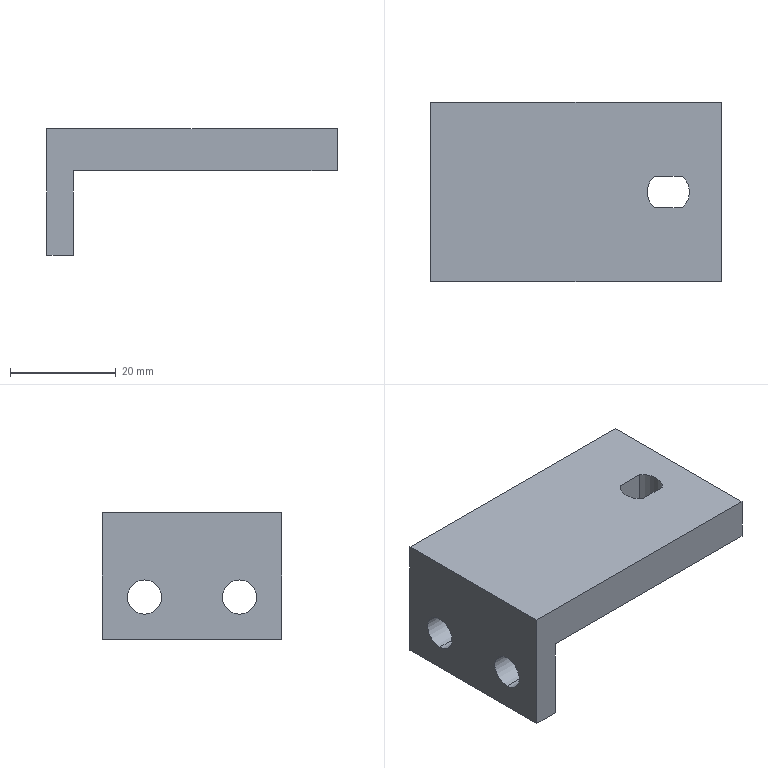Part | STEP file | 8xs043021 | 1 solid | 17 faces | box 55 x 34 x 24 mm | volume 17004 mm3 | plane 10 | cylinder 7 | commonest cylinder face diameters 6.5 x4 8 x3
STEP:
#1=CARTESIAN_POINT('',(0.,0.,0.));
#2=DIRECTION('',(0.,0.,1.));
#3=DIRECTION('',(1.,0.,0.));
#4=AXIS2_PLACEMENT_3D('',#1,#2,#3);
#5=CARTESIAN_POINT('',(14.854,3.,24.));
#6=VERTEX_POINT('',#5);
#7=CARTESIAN_POINT('',(14.854,3.,16.));
#8=VERTEX_POINT('',#7);
#9=CARTESIAN_POINT('',(14.854,3.,26.));
#10=DIRECTION('',(0.,0.,-1.));
#11=VECTOR('',#10,1.);
#12=LINE('',#9,#11);
#13=CARTESIAN_POINT('',(17.5,0.,26.));
#14=DIRECTION('',(0.,0.,-1.));
#15=DIRECTION('',(-1.,0.,0.));
#16=AXIS2_PLACEMENT_3D('',#13,#14,#15);
#17=CYLINDRICAL_SURFACE('',#16,4.);
#18=CARTESIAN_POINT('',(0.8481,0.));
#19=DIRECTION('',(0.,1.));
#20=VECTOR('',#19,1.);
#21=LINE('',#18,#20);
#22=(GEOMETRIC_REPRESENTATION_CONTEXT(2)PARAMETRIC_REPRESENTATION_CONTEXT()REPRESENTATION_CONTEXT('',''));
#23=DEFINITIONAL_REPRESENTATION('',(#21),#22);
#24=PCURVE('',#17,#23);
#25=CARTESIAN_POINT('',(20.146,3.,26.));
#26=DIRECTION('',(0.,1.,0.));
#27=DIRECTION('',(-1.,0.,0.));
#28=AXIS2_PLACEMENT_3D('',#25,#26,#27);
#29=PLANE('',#28);
#30=CARTESIAN_POINT('',(5.292,0.));
#31=DIRECTION('',(0.,-1.));
#32=VECTOR('',#31,1.);
#33=LINE('',#30,#32);
#34=(GEOMETRIC_REPRESENTATION_CONTEXT(2)PARAMETRIC_REPRESENTATION_CONTEXT()REPRESENTATION_CONTEXT('',''));
#35=DEFINITIONAL_REPRESENTATION('',(#33),#34);
#36=PCURVE('',#29,#35);
#37=SURFACE_CURVE('',#12,(#24,#36),.PCURVE_S1.);
#38=EDGE_CURVE('',#6,#8,#37,.T.);
#39=ORIENTED_EDGE('',*,*,#38,.T.);
#40=CARTESIAN_POINT('',(13.5,0.,16.));
#41=VERTEX_POINT('',#40);
#42=CARTESIAN_POINT('',(17.5,0.,16.));
#43=DIRECTION('',(0.,0.,-1.));
#44=DIRECTION('',(-1.,0.,0.));
#45=AXIS2_PLACEMENT_3D('',#42,#43,#44);
#46=CIRCLE('',#45,4.);
#47=CARTESIAN_POINT('',(0.,10.));
#48=DIRECTION('',(1.,0.));
#49=VECTOR('',#48,1.);
#50=LINE('',#47,#49);
#51=(GEOMETRIC_REPRESENTATION_CONTEXT(2)PARAMETRIC_REPRESENTATION_CONTEXT()REPRESENTATION_CONTEXT('',''));
#52=DEFINITIONAL_REPRESENTATION('',(#50),#51);
#53=PCURVE('',#17,#52);
#54=CARTESIAN_POINT('',(27.5,-17.,16.));
#55=DIRECTION('',(0.,0.,1.));
#56=DIRECTION('',(1.,0.,0.));
#57=AXIS2_PLACEMENT_3D('',#54,#55,#56);
#58=PLANE('',#57);
#59=CARTESIAN_POINT('',(-14.,17.));
#60=CARTESIAN_POINT('',(-14.,23.928));
#61=CARTESIAN_POINT('',(-8.,20.464));
#62=CARTESIAN_POINT('',(-2.,17.));
#63=CARTESIAN_POINT('',(-8.,13.536));
#64=CARTESIAN_POINT('',(-14.,10.072));
#65=CARTESIAN_POINT('',(-14.,17.));
#66=(BOUNDED_CURVE()B_SPLINE_CURVE(2,(#59,#60,#61,#62,#63,#64,#65),.UNSPECIFIED.,.T.,.F.)B_SPLINE_CURVE_WITH_KNOTS((1,2,2,2,2,1),(-2.094,0.,2.094,4.189,6.283,8.378),.UNSPECIFIED.)CURVE()GEOMETRIC_REPRESENTATION_ITEM()RATIONAL_B_SPLINE_CURVE((1.,0.5,1.,0.5,1.,0.5,1.))REPRESENTATION_ITEM(''));
#67=(GEOMETRIC_REPRESENTATION_CONTEXT(2)PARAMETRIC_REPRESENTATION_CONTEXT()REPRESENTATION_CONTEXT('',''));
#68=DEFINITIONAL_REPRESENTATION('',(#66),#67);
#69=PCURVE('',#58,#68);
#70=SURFACE_CURVE('',#46,(#53,#69),.PCURVE_S1.);
#71=EDGE_CURVE('',#41,#8,#70,.T.);
#72=ORIENTED_EDGE('',*,*,#71,.F.);
#73=CARTESIAN_POINT('',(13.5,0.,24.));
#74=VERTEX_POINT('',#73);
#75=CARTESIAN_POINT('',(13.5,0.,26.));
#76=DIRECTION('',(0.,0.,-1.));
#77=VECTOR('',#76,1.);
#78=LINE('',#75,#77);
#79=CARTESIAN_POINT('',(0.,0.));
#80=DIRECTION('',(0.,1.));
#81=VECTOR('',#80,1.);
#82=LINE('',#79,#81);
#83=(GEOMETRIC_REPRESENTATION_CONTEXT(2)PARAMETRIC_REPRESENTATION_CONTEXT()REPRESENTATION_CONTEXT('',''));
#84=DEFINITIONAL_REPRESENTATION('',(#82),#83);
#85=PCURVE('',#17,#84);
#86=CARTESIAN_POINT('',(17.5,0.,26.));
#87=DIRECTION('',(0.,0.,-1.));
#88=DIRECTION('',(-1.,0.,0.));
#89=AXIS2_PLACEMENT_3D('',#86,#87,#88);
#90=CYLINDRICAL_SURFACE('',#89,4.);
#91=CARTESIAN_POINT('',(6.283,0.));
#92=DIRECTION('',(0.,1.));
#93=VECTOR('',#92,1.);
#94=LINE('',#91,#93);
#95=(GEOMETRIC_REPRESENTATION_CONTEXT(2)PARAMETRIC_REPRESENTATION_CONTEXT()REPRESENTATION_CONTEXT('',''));
#96=DEFINITIONAL_REPRESENTATION('',(#94),#95);
#97=PCURVE('',#90,#96);
#98=SURFACE_CURVE('',#78,(#85,#97),.PCURVE_S1.);
#99=EDGE_CURVE('',#74,#41,#98,.T.);
#100=ORIENTED_EDGE('',*,*,#99,.F.);
#101=CARTESIAN_POINT('',(17.5,0.,24.));
#102=DIRECTION('',(0.,0.,-1.));
#103=DIRECTION('',(-1.,0.,0.));
#104=AXIS2_PLACEMENT_3D('',#101,#102,#103);
#105=CIRCLE('',#104,4.);
#106=CARTESIAN_POINT('',(0.,2.));
#107=DIRECTION('',(1.,0.));
#108=VECTOR('',#107,1.);
#109=LINE('',#106,#108);
#110=(GEOMETRIC_REPRESENTATION_CONTEXT(2)PARAMETRIC_REPRESENTATION_CONTEXT()REPRESENTATION_CONTEXT('',''));
#111=DEFINITIONAL_REPRESENTATION('',(#109),#110);
#112=PCURVE('',#17,#111);
#113=CARTESIAN_POINT('',(-27.5,-17.,24.));
#114=DIRECTION('',(0.,0.,-1.));
#115=DIRECTION('',(-1.,0.,0.));
#116=AXIS2_PLACEMENT_3D('',#113,#114,#115);
#117=PLANE('',#116);
#118=CARTESIAN_POINT('',(-45.,17.));
#119=DIRECTION('',(1.,0.));
#120=AXIS2_PLACEMENT_2D('',#118,#119);
#121=CIRCLE('',#120,4.);
#122=(GEOMETRIC_REPRESENTATION_CONTEXT(2)PARAMETRIC_REPRESENTATION_CONTEXT()REPRESENTATION_CONTEXT('',''));
#123=DEFINITIONAL_REPRESENTATION('',(#121),#122);
#124=PCURVE('',#117,#123);
#125=SURFACE_CURVE('',#105,(#112,#124),.PCURVE_S1.);
#126=EDGE_CURVE('',#74,#6,#125,.T.);
#127=ORIENTED_EDGE('',*,*,#126,.T.);
#128=EDGE_LOOP('',(#39,#72,#100,#127));
#129=FACE_BOUND('',#128,.F.);
#130=ADVANCED_FACE('',(#129),#17,.F.);
#131=CARTESIAN_POINT('',(-27.5,-9.,4.75));
#132=VERTEX_POINT('',#131);
#133=CARTESIAN_POINT('',(-22.5,-9.,4.75));
#134=VERTEX_POINT('',#133);
#135=CARTESIAN_POINT('',(-32.5,-9.,4.75));
#136=DIRECTION('',(1.,0.,0.));
#137=VECTOR('',#136,1.);
#138=LINE('',#135,#137);
#139=CARTESIAN_POINT('',(-32.5,-9.,8.));
#140=DIRECTION('',(1.,0.,0.));
#141=DIRECTION('',(0.,0.,-1.));
#142=AXIS2_PLACEMENT_3D('',#139,#140,#141);
#143=CYLINDRICAL_SURFACE('',#142,3.25);
#144=CARTESIAN_POINT('',(6.283,5.));
#145=CARTESIAN_POINT('',(6.283,5.076));
#146=CARTESIAN_POINT('',(6.283,5.227));
#147=CARTESIAN_POINT('',(6.283,5.455));
#148=CARTESIAN_POINT('',(6.283,5.682));
#149=CARTESIAN_POINT('',(6.283,5.909));
#150=CARTESIAN_POINT('',(6.283,6.136));
#151=CARTESIAN_POINT('',(6.283,6.364));
#152=CARTESIAN_POINT('',(6.283,6.591));
#153=CARTESIAN_POINT('',(6.283,6.818));
#154=CARTESIAN_POINT('',(6.283,7.045));
#155=CARTESIAN_POINT('',(6.283,7.273));
#156=CARTESIAN_POINT('',(6.283,7.5));
#157=CARTESIAN_POINT('',(6.283,7.727));
#158=CARTESIAN_POINT('',(6.283,7.955));
#159=CARTESIAN_POINT('',(6.283,8.182));
#160=CARTESIAN_POINT('',(6.283,8.409));
#161=CARTESIAN_POINT('',(6.283,8.636));
#162=CARTESIAN_POINT('',(6.283,8.864));
#163=CARTESIAN_POINT('',(6.283,9.091));
#164=CARTESIAN_POINT('',(6.283,9.318));
#165=CARTESIAN_POINT('',(6.283,9.545));
#166=CARTESIAN_POINT('',(6.283,9.773));
#167=CARTESIAN_POINT('',(6.283,9.924));
#168=CARTESIAN_POINT('',(6.283,10.));
#169=B_SPLINE_CURVE_WITH_KNOTS('',3,(#144,#145,#146,#147,#148,#149,#150,#151,#152,#153,#154,#155,#156,#157,#158,#159,#160,#161,#162,#163,#164,#165,#166,#167,#168),.UNSPECIFIED.,.F.,.F.,(4,1,1,1,1,1,1,1,1,1,1,1,1,1,1,1,1,1,1,1,1,1,4),(5.,5.227,5.455,5.682,5.909,6.136,6.364,6.591,6.818,7.045,7.273,7.5,7.727,7.955,8.182,8.409,8.636,8.864,9.091,9.318,9.545,9.773,10.),.QUASI_UNIFORM_KNOTS.);
#170=(GEOMETRIC_REPRESENTATION_CONTEXT(2)PARAMETRIC_REPRESENTATION_CONTEXT()REPRESENTATION_CONTEXT('',''));
#171=DEFINITIONAL_REPRESENTATION('',(#169),#170);
#172=PCURVE('',#143,#171);
#173=CARTESIAN_POINT('',(-32.5,-9.,8.));
#174=DIRECTION('',(1.,0.,0.));
#175=DIRECTION('',(0.,0.,-1.));
#176=AXIS2_PLACEMENT_3D('',#173,#174,#175);
#177=CYLINDRICAL_SURFACE('',#176,3.25);
#178=CARTESIAN_POINT('',(0.,0.));
#179=DIRECTION('',(0.,1.));
#180=VECTOR('',#179,1.);
#181=LINE('',#178,#180);
#182=(GEOMETRIC_REPRESENTATION_CONTEXT(2)PARAMETRIC_REPRESENTATION_CONTEXT()REPRESENTATION_CONTEXT('',''));
#183=DEFINITIONAL_REPRESENTATION('',(#181),#182);
#184=PCURVE('',#177,#183);
#185=SURFACE_CURVE('',#138,(#172,#184),.PCURVE_S1.);
#186=EDGE_CURVE('',#132,#134,#185,.T.);
#187=ORIENTED_EDGE('',*,*,#186,.T.);
#188=CARTESIAN_POINT('',(-22.5,-9.,11.25));
#189=VERTEX_POINT('',#188);
#190=CARTESIAN_POINT('',(-22.5,-9.,8.));
#191=DIRECTION('',(1.,0.,0.));
#192=DIRECTION('',(0.,0.,-1.));
#193=AXIS2_PLACEMENT_3D('',#190,#191,#192);
#194=CIRCLE('',#193,3.25);
#195=CARTESIAN_POINT('',(0.,10.));
#196=DIRECTION('',(1.,0.));
#197=VECTOR('',#196,1.);
#198=LINE('',#195,#197);
#199=(GEOMETRIC_REPRESENTATION_CONTEXT(2)PARAMETRIC_REPRESENTATION_CONTEXT()REPRESENTATION_CONTEXT('',''));
#200=DEFINITIONAL_REPRESENTATION('',(#198),#199);
#201=PCURVE('',#143,#200);
#202=CARTESIAN_POINT('',(-22.5,-17.,0.));
#203=DIRECTION('',(-1.,0.,0.));
#204=DIRECTION('',(0.,0.,1.));
#205=AXIS2_PLACEMENT_3D('',#202,#203,#204);
#206=PLANE('',#205);
#207=CARTESIAN_POINT('',(4.75,8.));
#208=CARTESIAN_POINT('',(4.75,13.629));
#209=CARTESIAN_POINT('',(9.625,10.815));
#210=CARTESIAN_POINT('',(14.5,8.));
#211=CARTESIAN_POINT('',(9.625,5.185));
#212=CARTESIAN_POINT('',(4.75,2.371));
#213=CARTESIAN_POINT('',(4.75,8.));
#214=(BOUNDED_CURVE()B_SPLINE_CURVE(2,(#207,#208,#209,#210,#211,#212,#213),.UNSPECIFIED.,.T.,.F.)B_SPLINE_CURVE_WITH_KNOTS((1,2,2,2,2,1),(-2.094,0.,2.094,4.189,6.283,8.378),.UNSPECIFIED.)CURVE()GEOMETRIC_REPRESENTATION_ITEM()RATIONAL_B_SPLINE_CURVE((1.,0.5,1.,0.5,1.,0.5,1.))REPRESENTATION_ITEM(''));
#215=(GEOMETRIC_REPRESENTATION_CONTEXT(2)PARAMETRIC_REPRESENTATION_CONTEXT()REPRESENTATION_CONTEXT('',''));
#216=DEFINITIONAL_REPRESENTATION('',(#214),#215);
#217=PCURVE('',#206,#216);
#218=SURFACE_CURVE('',#194,(#201,#217),.PCURVE_S1.);
#219=EDGE_CURVE('',#189,#134,#218,.T.);
#220=ORIENTED_EDGE('',*,*,#219,.F.);
#221=CARTESIAN_POINT('',(-27.5,-9.,11.25));
#222=VERTEX_POINT('',#221);
#223=CARTESIAN_POINT('',(-32.5,-9.,11.25));
#224=DIRECTION('',(1.,0.,0.));
#225=VECTOR('',#224,1.);
#226=LINE('',#223,#225);
#227=CARTESIAN_POINT('',(3.142,0.));
#228=DIRECTION('',(0.,1.));
#229=VECTOR('',#228,1.);
#230=LINE('',#227,#229);
#231=(GEOMETRIC_REPRESENTATION_CONTEXT(2)PARAMETRIC_REPRESENTATION_CONTEXT()REPRESENTATION_CONTEXT('',''));
#232=DEFINITIONAL_REPRESENTATION('',(#230),#231);
#233=PCURVE('',#143,#232);
#234=CARTESIAN_POINT('',(3.142,0.));
#235=DIRECTION('',(0.,1.));
#236=VECTOR('',#235,1.);
#237=LINE('',#234,#236);
#238=(GEOMETRIC_REPRESENTATION_CONTEXT(2)PARAMETRIC_REPRESENTATION_CONTEXT()REPRESENTATION_CONTEXT('',''));
#239=DEFINITIONAL_REPRESENTATION('',(#237),#238);
#240=PCURVE('',#177,#239);
#241=SURFACE_CURVE('',#226,(#233,#240),.PCURVE_S1.);
#242=EDGE_CURVE('',#222,#189,#241,.T.);
#243=ORIENTED_EDGE('',*,*,#242,.F.);
#244=CARTESIAN_POINT('',(-27.5,-9.,8.));
#245=DIRECTION('',(1.,0.,0.));
#246=DIRECTION('',(0.,1.,0.));
#247=AXIS2_PLACEMENT_3D('',#244,#245,#246);
#248=CIRCLE('',#247,3.25);
#249=CARTESIAN_POINT('',(1.571,5.));
#250=DIRECTION('',(1.,0.));
#251=VECTOR('',#250,1.);
#252=LINE('',#249,#251);
#253=(GEOMETRIC_REPRESENTATION_CONTEXT(2)PARAMETRIC_REPRESENTATION_CONTEXT()REPRESENTATION_CONTEXT('',''));
#254=DEFINITIONAL_REPRESENTATION('',(#252),#253);
#255=PCURVE('',#143,#254);
#256=CARTESIAN_POINT('',(-27.5,17.,24.));
#257=DIRECTION('',(1.,0.,0.));
#258=DIRECTION('',(0.,1.,0.));
#259=AXIS2_PLACEMENT_3D('',#256,#257,#258);
#260=PLANE('',#259);
#261=CARTESIAN_POINT('',(-26.,-16.));
#262=DIRECTION('',(1.,0.));
#263=AXIS2_PLACEMENT_2D('',#261,#262);
#264=CIRCLE('',#263,3.25);
#265=(GEOMETRIC_REPRESENTATION_CONTEXT(2)PARAMETRIC_REPRESENTATION_CONTEXT()REPRESENTATION_CONTEXT('',''));
#266=DEFINITIONAL_REPRESENTATION('',(#264),#265);
#267=PCURVE('',#260,#266);
#268=SURFACE_CURVE('',#248,(#255,#267),.PCURVE_S1.);
#269=EDGE_CURVE('',#222,#132,#268,.T.);
#270=ORIENTED_EDGE('',*,*,#269,.T.);
#271=EDGE_LOOP('',(#187,#220,#243,#270));
#272=FACE_BOUND('',#271,.F.);
#273=ADVANCED_FACE('',(#272),#143,.F.);
#274=CARTESIAN_POINT('',(-27.5,9.,4.75));
#275=VERTEX_POINT('',#274);
#276=CARTESIAN_POINT('',(-22.5,9.,4.75));
#277=VERTEX_POINT('',#276);
#278=CARTESIAN_POINT('',(-32.5,9.,4.75));
#279=DIRECTION('',(1.,0.,0.));
#280=VECTOR('',#279,1.);
#281=LINE('',#278,#280);
#282=CARTESIAN_POINT('',(-32.5,9.,8.));
#283=DIRECTION('',(1.,0.,0.));
#284=DIRECTION('',(0.,0.,-1.));
#285=AXIS2_PLACEMENT_3D('',#282,#283,#284);
#286=CYLINDRICAL_SURFACE('',#285,3.25);
#287=CARTESIAN_POINT('',(6.283,5.));
#288=CARTESIAN_POINT('',(6.283,5.076));
#289=CARTESIAN_POINT('',(6.283,5.227));
#290=CARTESIAN_POINT('',(6.283,5.455));
#291=CARTESIAN_POINT('',(6.283,5.682));
#292=CARTESIAN_POINT('',(6.283,5.909));
#293=CARTESIAN_POINT('',(6.283,6.136));
#294=CARTESIAN_POINT('',(6.283,6.364));
#295=CARTESIAN_POINT('',(6.283,6.591));
#296=CARTESIAN_POINT('',(6.283,6.818));
#297=CARTESIAN_POINT('',(6.283,7.045));
#298=CARTESIAN_POINT('',(6.283,7.273));
#299=CARTESIAN_POINT('',(6.283,7.5));
#300=CARTESIAN_POINT('',(6.283,7.727));
#301=CARTESIAN_POINT('',(6.283,7.955));
#302=CARTESIAN_POINT('',(6.283,8.182));
#303=CARTESIAN_POINT('',(6.283,8.409));
#304=CARTESIAN_POINT('',(6.283,8.636));
#305=CARTESIAN_POINT('',(6.283,8.864));
#306=CARTESIAN_POINT('',(6.283,9.091));
#307=CARTESIAN_POINT('',(6.283,9.318));
#308=CARTESIAN_POINT('',(6.283,9.545));
#309=CARTESIAN_POINT('',(6.283,9.773));
#310=CARTESIAN_POINT('',(6.283,9.924));
#311=CARTESIAN_POINT('',(6.283,10.));
#312=B_SPLINE_CURVE_WITH_KNOTS('',3,(#287,#288,#289,#290,#291,#292,#293,#294,#295,#296,#297,#298,#299,#300,#301,#302,#303,#304,#305,#306,#307,#308,#309,#310,#311),.UNSPECIFIED.,.F.,.F.,(4,1,1,1,1,1,1,1,1,1,1,1,1,1,1,1,1,1,1,1,1,1,4),(5.,5.227,5.455,5.682,5.909,6.136,6.364,6.591,6.818,7.045,7.273,7.5,7.727,7.955,8.182,8.409,8.636,8.864,9.091,9.318,9.545,9.773,10.),.QUASI_UNIFORM_KNOTS.);
#313=(GEOMETRIC_REPRESENTATION_CONTEXT(2)PARAMETRIC_REPRESENTATION_CONTEXT()REPRESENTATION_CONTEXT('',''));
#314=DEFINITIONAL_REPRESENTATION('',(#312),#313);
#315=PCURVE('',#286,#314);
#316=CARTESIAN_POINT('',(-32.5,9.,8.));
#317=DIRECTION('',(1.,0.,0.));
#318=DIRECTION('',(0.,0.,-1.));
#319=AXIS2_PLACEMENT_3D('',#316,#317,#318);
#320=CYLINDRICAL_SURFACE('',#319,3.25);
#321=CARTESIAN_POINT('',(0.,0.));
#322=DIRECTION('',(0.,1.));
#323=VECTOR('',#322,1.);
#324=LINE('',#321,#323);
#325=(GEOMETRIC_REPRESENTATION_CONTEXT(2)PARAMETRIC_REPRESENTATION_CONTEXT()REPRESENTATION_CONTEXT('',''));
#326=DEFINITIONAL_REPRESENTATION('',(#324),#325);
#327=PCURVE('',#320,#326);
#328=SURFACE_CURVE('',#281,(#315,#327),.PCURVE_S1.);
#329=EDGE_CURVE('',#275,#277,#328,.T.);
#330=ORIENTED_EDGE('',*,*,#329,.T.);
#331=CARTESIAN_POINT('',(-22.5,9.,11.25));
#332=VERTEX_POINT('',#331);
#333=CARTESIAN_POINT('',(-22.5,9.,8.));
#334=DIRECTION('',(1.,0.,0.));
#335=DIRECTION('',(0.,0.,-1.));
#336=AXIS2_PLACEMENT_3D('',#333,#334,#335);
#337=CIRCLE('',#336,3.25);
#338=CARTESIAN_POINT('',(0.,10.));
#339=DIRECTION('',(1.,0.));
#340=VECTOR('',#339,1.);
#341=LINE('',#338,#340);
#342=(GEOMETRIC_REPRESENTATION_CONTEXT(2)PARAMETRIC_REPRESENTATION_CONTEXT()REPRESENTATION_CONTEXT('',''));
#343=DEFINITIONAL_REPRESENTATION('',(#341),#342);
#344=PCURVE('',#286,#343);
#345=CARTESIAN_POINT('',(4.75,26.));
#346=CARTESIAN_POINT('',(4.75,31.629));
#347=CARTESIAN_POINT('',(9.625,28.815));
#348=CARTESIAN_POINT('',(14.5,26.));
#349=CARTESIAN_POINT('',(9.625,23.185));
#350=CARTESIAN_POINT('',(4.75,20.371));
#351=CARTESIAN_POINT('',(4.75,26.));
#352=(BOUNDED_CURVE()B_SPLINE_CURVE(2,(#345,#346,#347,#348,#349,#350,#351),.UNSPECIFIED.,.T.,.F.)B_SPLINE_CURVE_WITH_KNOTS((1,2,2,2,2,1),(-2.094,0.,2.094,4.189,6.283,8.378),.UNSPECIFIED.)CURVE()GEOMETRIC_REPRESENTATION_ITEM()RATIONAL_B_SPLINE_CURVE((1.,0.5,1.,0.5,1.,0.5,1.))REPRESENTATION_ITEM(''));
#353=(GEOMETRIC_REPRESENTATION_CONTEXT(2)PARAMETRIC_REPRESENTATION_CONTEXT()REPRESENTATION_CONTEXT('',''));
#354=DEFINITIONAL_REPRESENTATION('',(#352),#353);
#355=PCURVE('',#206,#354);
#356=SURFACE_CURVE('',#337,(#344,#355),.PCURVE_S1.);
#357=EDGE_CURVE('',#332,#277,#356,.T.);
#358=ORIENTED_EDGE('',*,*,#357,.F.);
#359=CARTESIAN_POINT('',(-27.5,9.,11.25));
#360=VERTEX_POINT('',#359);
#361=CARTESIAN_POINT('',(-32.5,9.,11.25));
#362=DIRECTION('',(1.,0.,0.));
#363=VECTOR('',#362,1.);
#364=LINE('',#361,#363);
#365=CARTESIAN_POINT('',(3.142,0.));
#366=DIRECTION('',(0.,1.));
#367=VECTOR('',#366,1.);
#368=LINE('',#365,#367);
#369=(GEOMETRIC_REPRESENTATION_CONTEXT(2)PARAMETRIC_REPRESENTATION_CONTEXT()REPRESENTATION_CONTEXT('',''));
#370=DEFINITIONAL_REPRESENTATION('',(#368),#369);
#371=PCURVE('',#286,#370);
#372=CARTESIAN_POINT('',(3.142,0.));
#373=DIRECTION('',(0.,1.));
#374=VECTOR('',#373,1.);
#375=LINE('',#372,#374);
#376=(GEOMETRIC_REPRESENTATION_CONTEXT(2)PARAMETRIC_REPRESENTATION_CONTEXT()REPRESENTATION_CONTEXT('',''));
#377=DEFINITIONAL_REPRESENTATION('',(#375),#376);
#378=PCURVE('',#320,#377);
#379=SURFACE_CURVE('',#364,(#371,#378),.PCURVE_S1.);
#380=EDGE_CURVE('',#360,#332,#379,.T.);
#381=ORIENTED_EDGE('',*,*,#380,.F.);
#382=CARTESIAN_POINT('',(-27.5,9.,8.));
#383=DIRECTION('',(1.,0.,0.));
#384=DIRECTION('',(0.,1.,0.));
#385=AXIS2_PLACEMENT_3D('',#382,#383,#384);
#386=CIRCLE('',#385,3.25);
#387=CARTESIAN_POINT('',(1.571,5.));
#388=DIRECTION('',(1.,0.));
#389=VECTOR('',#388,1.);
#390=LINE('',#387,#389);
#391=(GEOMETRIC_REPRESENTATION_CONTEXT(2)PARAMETRIC_REPRESENTATION_CONTEXT()REPRESENTATION_CONTEXT('',''));
#392=DEFINITIONAL_REPRESENTATION('',(#390),#391);
#393=PCURVE('',#286,#392);
#394=CARTESIAN_POINT('',(-8.,-16.));
#395=DIRECTION('',(1.,0.));
#396=AXIS2_PLACEMENT_2D('',#394,#395);
#397=CIRCLE('',#396,3.25);
#398=(GEOMETRIC_REPRESENTATION_CONTEXT(2)PARAMETRIC_REPRESENTATION_CONTEXT()REPRESENTATION_CONTEXT('',''));
#399=DEFINITIONAL_REPRESENTATION('',(#397),#398);
#400=PCURVE('',#260,#399);
#401=SURFACE_CURVE('',#386,(#393,#400),.PCURVE_S1.);
#402=EDGE_CURVE('',#360,#275,#401,.T.);
#403=ORIENTED_EDGE('',*,*,#402,.T.);
#404=EDGE_LOOP('',(#330,#358,#381,#403));
#405=FACE_BOUND('',#404,.F.);
#406=ADVANCED_FACE('',(#405),#286,.F.);
#407=CARTESIAN_POINT('',(-27.5,-9.,8.));
#408=DIRECTION('',(1.,0.,0.));
#409=DIRECTION('',(0.,1.,0.));
#410=AXIS2_PLACEMENT_3D('',#407,#408,#409);
#411=CIRCLE('',#410,3.25);
#412=CARTESIAN_POINT('',(-26.,-16.));
#413=DIRECTION('',(1.,0.));
#414=AXIS2_PLACEMENT_2D('',#412,#413);
#415=CIRCLE('',#414,3.25);
#416=(GEOMETRIC_REPRESENTATION_CONTEXT(2)PARAMETRIC_REPRESENTATION_CONTEXT()REPRESENTATION_CONTEXT('',''));
#417=DEFINITIONAL_REPRESENTATION('',(#415),#416);
#418=PCURVE('',#260,#417);
#419=CARTESIAN_POINT('',(-4.712,5.));
#420=DIRECTION('',(1.,0.));
#421=VECTOR('',#420,1.);
#422=LINE('',#419,#421);
#423=(GEOMETRIC_REPRESENTATION_CONTEXT(2)PARAMETRIC_REPRESENTATION_CONTEXT()REPRESENTATION_CONTEXT('',''));
#424=DEFINITIONAL_REPRESENTATION('',(#422),#423);
#425=PCURVE('',#177,#424);
#426=SURFACE_CURVE('',#411,(#418,#425),.PCURVE_S1.);
#427=EDGE_CURVE('',#132,#222,#426,.T.);
#428=ORIENTED_EDGE('',*,*,#427,.T.);
#429=ORIENTED_EDGE('',*,*,#269,.T.);
#430=EDGE_LOOP('',(#428,#429));
#431=FACE_BOUND('',#430,.T.);
#432=CARTESIAN_POINT('',(-27.5,9.,8.));
#433=DIRECTION('',(1.,0.,0.));
#434=DIRECTION('',(0.,1.,0.));
#435=AXIS2_PLACEMENT_3D('',#432,#433,#434);
#436=CIRCLE('',#435,3.25);
#437=CARTESIAN_POINT('',(-8.,-16.));
#438=DIRECTION('',(1.,0.));
#439=AXIS2_PLACEMENT_2D('',#437,#438);
#440=CIRCLE('',#439,3.25);
#441=(GEOMETRIC_REPRESENTATION_CONTEXT(2)PARAMETRIC_REPRESENTATION_CONTEXT()REPRESENTATION_CONTEXT('',''));
#442=DEFINITIONAL_REPRESENTATION('',(#440),#441);
#443=PCURVE('',#260,#442);
#444=CARTESIAN_POINT('',(-4.712,5.));
#445=DIRECTION('',(1.,0.));
#446=VECTOR('',#445,1.);
#447=LINE('',#444,#446);
#448=(GEOMETRIC_REPRESENTATION_CONTEXT(2)PARAMETRIC_REPRESENTATION_CONTEXT()REPRESENTATION_CONTEXT('',''));
#449=DEFINITIONAL_REPRESENTATION('',(#447),#448);
#450=PCURVE('',#320,#449);
#451=SURFACE_CURVE('',#436,(#443,#450),.PCURVE_S1.);
#452=EDGE_CURVE('',#275,#360,#451,.T.);
#453=ORIENTED_EDGE('',*,*,#452,.T.);
#454=ORIENTED_EDGE('',*,*,#402,.T.);
#455=EDGE_LOOP('',(#453,#454));
#456=FACE_BOUND('',#455,.T.);
#457=CARTESIAN_POINT('',(-27.5,17.,0.));
#458=VERTEX_POINT('',#457);
#459=CARTESIAN_POINT('',(-27.5,-17.,0.));
#460=VERTEX_POINT('',#459);
#461=CARTESIAN_POINT('',(-27.5,17.,0.));
#462=DIRECTION('',(0.,-1.,0.));
#463=VECTOR('',#462,1.);
#464=LINE('',#461,#463);
#465=CARTESIAN_POINT('',(0.,-24.));
#466=DIRECTION('',(-1.,0.));
#467=VECTOR('',#466,1.);
#468=LINE('',#465,#467);
#469=(GEOMETRIC_REPRESENTATION_CONTEXT(2)PARAMETRIC_REPRESENTATION_CONTEXT()REPRESENTATION_CONTEXT('',''));
#470=DEFINITIONAL_REPRESENTATION('',(#468),#469);
#471=PCURVE('',#260,#470);
#472=CARTESIAN_POINT('',(-27.5,-17.,0.));
#473=DIRECTION('',(0.,0.,-1.));
#474=DIRECTION('',(-1.,0.,0.));
#475=AXIS2_PLACEMENT_3D('',#472,#473,#474);
#476=PLANE('',#475);
#477=CARTESIAN_POINT('',(0.,34.));
#478=DIRECTION('',(0.,-1.));
#479=VECTOR('',#478,1.);
#480=LINE('',#477,#479);
#481=(GEOMETRIC_REPRESENTATION_CONTEXT(2)PARAMETRIC_REPRESENTATION_CONTEXT()REPRESENTATION_CONTEXT('',''));
#482=DEFINITIONAL_REPRESENTATION('',(#480),#481);
#483=PCURVE('',#476,#482);
#484=SURFACE_CURVE('',#464,(#471,#483),.PCURVE_S1.);
#485=EDGE_CURVE('',#458,#460,#484,.T.);
#486=ORIENTED_EDGE('',*,*,#485,.T.);
#487=CARTESIAN_POINT('',(-27.5,-17.,24.));
#488=VERTEX_POINT('',#487);
#489=CARTESIAN_POINT('',(-27.5,-17.,24.));
#490=DIRECTION('',(0.,0.,-1.));
#491=VECTOR('',#490,1.);
#492=LINE('',#489,#491);
#493=CARTESIAN_POINT('',(-34.,0.));
#494=DIRECTION('',(0.,-1.));
#495=VECTOR('',#494,1.);
#496=LINE('',#493,#495);
#497=(GEOMETRIC_REPRESENTATION_CONTEXT(2)PARAMETRIC_REPRESENTATION_CONTEXT()REPRESENTATION_CONTEXT('',''));
#498=DEFINITIONAL_REPRESENTATION('',(#496),#497);
#499=PCURVE('',#260,#498);
#500=CARTESIAN_POINT('',(27.5,-17.,24.));
#501=DIRECTION('',(0.,1.,0.));
#502=DIRECTION('',(-1.,0.,0.));
#503=AXIS2_PLACEMENT_3D('',#500,#501,#502);
#504=PLANE('',#503);
#505=CARTESIAN_POINT('',(55.,0.));
#506=DIRECTION('',(0.,-1.));
#507=VECTOR('',#506,1.);
#508=LINE('',#505,#507);
#509=(GEOMETRIC_REPRESENTATION_CONTEXT(2)PARAMETRIC_REPRESENTATION_CONTEXT()REPRESENTATION_CONTEXT('',''));
#510=DEFINITIONAL_REPRESENTATION('',(#508),#509);
#511=PCURVE('',#504,#510);
#512=SURFACE_CURVE('',#492,(#499,#511),.PCURVE_S1.);
#513=EDGE_CURVE('',#488,#460,#512,.T.);
#514=ORIENTED_EDGE('',*,*,#513,.F.);
#515=CARTESIAN_POINT('',(-27.5,17.,24.));
#516=VERTEX_POINT('',#515);
#517=CARTESIAN_POINT('',(-27.5,17.,24.));
#518=DIRECTION('',(0.,-1.,0.));
#519=VECTOR('',#518,1.);
#520=LINE('',#517,#519);
#521=CARTESIAN_POINT('',(0.,0.));
#522=DIRECTION('',(-1.,0.));
#523=VECTOR('',#522,1.);
#524=LINE('',#521,#523);
#525=(GEOMETRIC_REPRESENTATION_CONTEXT(2)PARAMETRIC_REPRESENTATION_CONTEXT()REPRESENTATION_CONTEXT('',''));
#526=DEFINITIONAL_REPRESENTATION('',(#524),#525);
#527=PCURVE('',#260,#526);
#528=CARTESIAN_POINT('',(0.,34.));
#529=DIRECTION('',(0.,-1.));
#530=VECTOR('',#529,1.);
#531=LINE('',#528,#530);
#532=(GEOMETRIC_REPRESENTATION_CONTEXT(2)PARAMETRIC_REPRESENTATION_CONTEXT()REPRESENTATION_CONTEXT('',''));
#533=DEFINITIONAL_REPRESENTATION('',(#531),#532);
#534=PCURVE('',#117,#533);
#535=SURFACE_CURVE('',#520,(#527,#534),.PCURVE_S1.);
#536=EDGE_CURVE('',#516,#488,#535,.T.);
#537=ORIENTED_EDGE('',*,*,#536,.F.);
#538=CARTESIAN_POINT('',(-27.5,17.,24.));
#539=DIRECTION('',(0.,0.,-1.));
#540=VECTOR('',#539,1.);
#541=LINE('',#538,#540);
#542=CARTESIAN_POINT('',(0.,0.));
#543=DIRECTION('',(0.,-1.));
#544=VECTOR('',#543,1.);
#545=LINE('',#542,#544);
#546=(GEOMETRIC_REPRESENTATION_CONTEXT(2)PARAMETRIC_REPRESENTATION_CONTEXT()REPRESENTATION_CONTEXT('',''));
#547=DEFINITIONAL_REPRESENTATION('',(#545),#546);
#548=PCURVE('',#260,#547);
#549=CARTESIAN_POINT('',(27.5,17.,24.));
#550=DIRECTION('',(0.,-1.,0.));
#551=DIRECTION('',(1.,0.,0.));
#552=AXIS2_PLACEMENT_3D('',#549,#550,#551);
#553=PLANE('',#552);
#554=CARTESIAN_POINT('',(-55.,0.));
#555=DIRECTION('',(0.,-1.));
#556=VECTOR('',#555,1.);
#557=LINE('',#554,#556);
#558=(GEOMETRIC_REPRESENTATION_CONTEXT(2)PARAMETRIC_REPRESENTATION_CONTEXT()REPRESENTATION_CONTEXT('',''));
#559=DEFINITIONAL_REPRESENTATION('',(#557),#558);
#560=PCURVE('',#553,#559);
#561=SURFACE_CURVE('',#541,(#548,#560),.PCURVE_S1.);
#562=EDGE_CURVE('',#516,#458,#561,.T.);
#563=ORIENTED_EDGE('',*,*,#562,.T.);
#564=EDGE_LOOP('',(#486,#514,#537,#563));
#565=FACE_BOUND('',#564,.T.);
#566=ADVANCED_FACE('',(#431,#456,#565),#260,.F.);
#567=CARTESIAN_POINT('',(-22.5,-17.,0.));
#568=VERTEX_POINT('',#567);
#569=CARTESIAN_POINT('',(-22.5,-17.,16.));
#570=VERTEX_POINT('',#569);
#571=CARTESIAN_POINT('',(-22.5,-17.,0.));
#572=DIRECTION('',(0.,0.,1.));
#573=VECTOR('',#572,1.);
#574=LINE('',#571,#573);
#575=CARTESIAN_POINT('',(50.,-24.));
#576=DIRECTION('',(0.,1.));
#577=VECTOR('',#576,1.);
#578=LINE('',#575,#577);
#579=(GEOMETRIC_REPRESENTATION_CONTEXT(2)PARAMETRIC_REPRESENTATION_CONTEXT()REPRESENTATION_CONTEXT('',''));
#580=DEFINITIONAL_REPRESENTATION('',(#578),#579);
#581=PCURVE('',#504,#580);
#582=CARTESIAN_POINT('',(0.,0.));
#583=DIRECTION('',(1.,0.));
#584=VECTOR('',#583,1.);
#585=LINE('',#582,#584);
#586=(GEOMETRIC_REPRESENTATION_CONTEXT(2)PARAMETRIC_REPRESENTATION_CONTEXT()REPRESENTATION_CONTEXT('',''));
#587=DEFINITIONAL_REPRESENTATION('',(#585),#586);
#588=PCURVE('',#206,#587);
#589=SURFACE_CURVE('',#574,(#581,#588),.PCURVE_S1.);
#590=EDGE_CURVE('',#568,#570,#589,.T.);
#591=ORIENTED_EDGE('',*,*,#590,.T.);
#592=CARTESIAN_POINT('',(27.5,-17.,16.));
#593=VERTEX_POINT('',#592);
#594=CARTESIAN_POINT('',(27.5,-17.,16.));
#595=DIRECTION('',(1.,0.,0.));
#596=VECTOR('',#595,1.);
#597=LINE('',#594,#596);
#598=CARTESIAN_POINT('',(0.,-8.));
#599=DIRECTION('',(-1.,0.));
#600=VECTOR('',#599,1.);
#601=LINE('',#598,#600);
#602=(GEOMETRIC_REPRESENTATION_CONTEXT(2)PARAMETRIC_REPRESENTATION_CONTEXT()REPRESENTATION_CONTEXT('',''));
#603=DEFINITIONAL_REPRESENTATION('',(#601),#602);
#604=PCURVE('',#504,#603);
#605=CARTESIAN_POINT('',(0.,0.));
#606=DIRECTION('',(1.,0.));
#607=VECTOR('',#606,1.);
#608=LINE('',#605,#607);
#609=(GEOMETRIC_REPRESENTATION_CONTEXT(2)PARAMETRIC_REPRESENTATION_CONTEXT()REPRESENTATION_CONTEXT('',''));
#610=DEFINITIONAL_REPRESENTATION('',(#608),#609);
#611=PCURVE('',#58,#610);
#612=SURFACE_CURVE('',#597,(#604,#611),.PCURVE_S1.);
#613=EDGE_CURVE('',#570,#593,#612,.T.);
#614=ORIENTED_EDGE('',*,*,#613,.T.);
#615=CARTESIAN_POINT('',(27.5,-17.,24.));
#616=VERTEX_POINT('',#615);
#617=CARTESIAN_POINT('',(27.5,-17.,24.));
#618=DIRECTION('',(0.,0.,-1.));
#619=VECTOR('',#618,1.);
#620=LINE('',#617,#619);
#621=CARTESIAN_POINT('',(0.,0.));
#622=DIRECTION('',(0.,-1.));
#623=VECTOR('',#622,1.);
#624=LINE('',#621,#623);
#625=(GEOMETRIC_REPRESENTATION_CONTEXT(2)PARAMETRIC_REPRESENTATION_CONTEXT()REPRESENTATION_CONTEXT('',''));
#626=DEFINITIONAL_REPRESENTATION('',(#624),#625);
#627=PCURVE('',#504,#626);
#628=CARTESIAN_POINT('',(27.5,17.,24.));
#629=DIRECTION('',(-1.,0.,0.));
#630=DIRECTION('',(0.,-1.,0.));
#631=AXIS2_PLACEMENT_3D('',#628,#629,#630);
#632=PLANE('',#631);
#633=CARTESIAN_POINT('',(34.,0.));
#634=DIRECTION('',(0.,-1.));
#635=VECTOR('',#634,1.);
#636=LINE('',#633,#635);
#637=(GEOMETRIC_REPRESENTATION_CONTEXT(2)PARAMETRIC_REPRESENTATION_CONTEXT()REPRESENTATION_CONTEXT('',''));
#638=DEFINITIONAL_REPRESENTATION('',(#636),#637);
#639=PCURVE('',#632,#638);
#640=SURFACE_CURVE('',#620,(#627,#639),.PCURVE_S1.);
#641=EDGE_CURVE('',#616,#593,#640,.T.);
#642=ORIENTED_EDGE('',*,*,#641,.F.);
#643=CARTESIAN_POINT('',(27.5,-17.,24.));
#644=DIRECTION('',(1.,0.,0.));
#645=VECTOR('',#644,1.);
#646=LINE('',#643,#645);
#647=CARTESIAN_POINT('',(0.,0.));
#648=DIRECTION('',(-1.,0.));
#649=VECTOR('',#648,1.);
#650=LINE('',#647,#649);
#651=(GEOMETRIC_REPRESENTATION_CONTEXT(2)PARAMETRIC_REPRESENTATION_CONTEXT()REPRESENTATION_CONTEXT('',''));
#652=DEFINITIONAL_REPRESENTATION('',(#650),#651);
#653=PCURVE('',#504,#652);
#654=CARTESIAN_POINT('',(-55.,0.));
#655=DIRECTION('',(-1.,0.));
#656=VECTOR('',#655,1.);
#657=LINE('',#654,#656);
#658=(GEOMETRIC_REPRESENTATION_CONTEXT(2)PARAMETRIC_REPRESENTATION_CONTEXT()REPRESENTATION_CONTEXT('',''));
#659=DEFINITIONAL_REPRESENTATION('',(#657),#658);
#660=PCURVE('',#117,#659);
#661=SURFACE_CURVE('',#646,(#653,#660),.PCURVE_S1.);
#662=EDGE_CURVE('',#488,#616,#661,.T.);
#663=ORIENTED_EDGE('',*,*,#662,.F.);
#664=ORIENTED_EDGE('',*,*,#513,.T.);
#665=CARTESIAN_POINT('',(27.5,-17.,0.));
#666=DIRECTION('',(1.,0.,0.));
#667=VECTOR('',#666,1.);
#668=LINE('',#665,#667);
#669=CARTESIAN_POINT('',(0.,-24.));
#670=DIRECTION('',(-1.,0.));
#671=VECTOR('',#670,1.);
#672=LINE('',#669,#671);
#673=(GEOMETRIC_REPRESENTATION_CONTEXT(2)PARAMETRIC_REPRESENTATION_CONTEXT()REPRESENTATION_CONTEXT('',''));
#674=DEFINITIONAL_REPRESENTATION('',(#672),#673);
#675=PCURVE('',#504,#674);
#676=CARTESIAN_POINT('',(-55.,0.));
#677=DIRECTION('',(-1.,0.));
#678=VECTOR('',#677,1.);
#679=LINE('',#676,#678);
#680=(GEOMETRIC_REPRESENTATION_CONTEXT(2)PARAMETRIC_REPRESENTATION_CONTEXT()REPRESENTATION_CONTEXT('',''));
#681=DEFINITIONAL_REPRESENTATION('',(#679),#680);
#682=PCURVE('',#476,#681);
#683=SURFACE_CURVE('',#668,(#675,#682),.PCURVE_S1.);
#684=EDGE_CURVE('',#460,#568,#683,.T.);
#685=ORIENTED_EDGE('',*,*,#684,.T.);
#686=EDGE_LOOP('',(#591,#614,#642,#663,#664,#685));
#687=FACE_BOUND('',#686,.T.);
#688=ADVANCED_FACE('',(#687),#504,.F.);
#689=ORIENTED_EDGE('',*,*,#641,.T.);
#690=CARTESIAN_POINT('',(27.5,17.,16.));
#691=VERTEX_POINT('',#690);
#692=CARTESIAN_POINT('',(27.5,-17.,16.));
#693=DIRECTION('',(0.,1.,0.));
#694=VECTOR('',#693,1.);
#695=LINE('',#692,#694);
#696=CARTESIAN_POINT('',(34.,-8.));
#697=DIRECTION('',(-1.,0.));
#698=VECTOR('',#697,1.);
#699=LINE('',#696,#698);
#700=(GEOMETRIC_REPRESENTATION_CONTEXT(2)PARAMETRIC_REPRESENTATION_CONTEXT()REPRESENTATION_CONTEXT('',''));
#701=DEFINITIONAL_REPRESENTATION('',(#699),#700);
#702=PCURVE('',#632,#701);
#703=CARTESIAN_POINT('',(0.,0.));
#704=DIRECTION('',(0.,1.));
#705=VECTOR('',#704,1.);
#706=LINE('',#703,#705);
#707=(GEOMETRIC_REPRESENTATION_CONTEXT(2)PARAMETRIC_REPRESENTATION_CONTEXT()REPRESENTATION_CONTEXT('',''));
#708=DEFINITIONAL_REPRESENTATION('',(#706),#707);
#709=PCURVE('',#58,#708);
#710=SURFACE_CURVE('',#695,(#702,#709),.PCURVE_S1.);
#711=EDGE_CURVE('',#593,#691,#710,.T.);
#712=ORIENTED_EDGE('',*,*,#711,.T.);
#713=CARTESIAN_POINT('',(27.5,17.,24.));
#714=VERTEX_POINT('',#713);
#715=CARTESIAN_POINT('',(27.5,17.,24.));
#716=DIRECTION('',(0.,0.,-1.));
#717=VECTOR('',#716,1.);
#718=LINE('',#715,#717);
#719=CARTESIAN_POINT('',(0.,0.));
#720=DIRECTION('',(0.,-1.));
#721=VECTOR('',#720,1.);
#722=LINE('',#719,#721);
#723=(GEOMETRIC_REPRESENTATION_CONTEXT(2)PARAMETRIC_REPRESENTATION_CONTEXT()REPRESENTATION_CONTEXT('',''));
#724=DEFINITIONAL_REPRESENTATION('',(#722),#723);
#725=PCURVE('',#632,#724);
#726=CARTESIAN_POINT('',(0.,0.));
#727=DIRECTION('',(0.,-1.));
#728=VECTOR('',#727,1.);
#729=LINE('',#726,#728);
#730=(GEOMETRIC_REPRESENTATION_CONTEXT(2)PARAMETRIC_REPRESENTATION_CONTEXT()REPRESENTATION_CONTEXT('',''));
#731=DEFINITIONAL_REPRESENTATION('',(#729),#730);
#732=PCURVE('',#553,#731);
#733=SURFACE_CURVE('',#718,(#725,#732),.PCURVE_S1.);
#734=EDGE_CURVE('',#714,#691,#733,.T.);
#735=ORIENTED_EDGE('',*,*,#734,.F.);
#736=CARTESIAN_POINT('',(27.5,17.,24.));
#737=DIRECTION('',(0.,1.,0.));
#738=VECTOR('',#737,1.);
#739=LINE('',#736,#738);
#740=CARTESIAN_POINT('',(0.,0.));
#741=DIRECTION('',(-1.,0.));
#742=VECTOR('',#741,1.);
#743=LINE('',#740,#742);
#744=(GEOMETRIC_REPRESENTATION_CONTEXT(2)PARAMETRIC_REPRESENTATION_CONTEXT()REPRESENTATION_CONTEXT('',''));
#745=DEFINITIONAL_REPRESENTATION('',(#743),#744);
#746=PCURVE('',#632,#745);
#747=CARTESIAN_POINT('',(-55.,34.));
#748=DIRECTION('',(0.,1.));
#749=VECTOR('',#748,1.);
#750=LINE('',#747,#749);
#751=(GEOMETRIC_REPRESENTATION_CONTEXT(2)PARAMETRIC_REPRESENTATION_CONTEXT()REPRESENTATION_CONTEXT('',''));
#752=DEFINITIONAL_REPRESENTATION('',(#750),#751);
#753=PCURVE('',#117,#752);
#754=SURFACE_CURVE('',#739,(#746,#753),.PCURVE_S1.);
#755=EDGE_CURVE('',#616,#714,#754,.T.);
#756=ORIENTED_EDGE('',*,*,#755,.F.);
#757=EDGE_LOOP('',(#689,#712,#735,#756));
#758=FACE_BOUND('',#757,.T.);
#759=ADVANCED_FACE('',(#758),#632,.F.);
#760=ORIENTED_EDGE('',*,*,#734,.T.);
#761=CARTESIAN_POINT('',(-22.5,17.,16.));
#762=VERTEX_POINT('',#761);
#763=CARTESIAN_POINT('',(27.5,17.,16.));
#764=DIRECTION('',(1.,0.,0.));
#765=VECTOR('',#764,1.);
#766=LINE('',#763,#765);
#767=CARTESIAN_POINT('',(0.,-8.));
#768=DIRECTION('',(1.,0.));
#769=VECTOR('',#768,1.);
#770=LINE('',#767,#769);
#771=(GEOMETRIC_REPRESENTATION_CONTEXT(2)PARAMETRIC_REPRESENTATION_CONTEXT()REPRESENTATION_CONTEXT('',''));
#772=DEFINITIONAL_REPRESENTATION('',(#770),#771);
#773=PCURVE('',#553,#772);
#774=CARTESIAN_POINT('',(0.,34.));
#775=DIRECTION('',(1.,0.));
#776=VECTOR('',#775,1.);
#777=LINE('',#774,#776);
#778=(GEOMETRIC_REPRESENTATION_CONTEXT(2)PARAMETRIC_REPRESENTATION_CONTEXT()REPRESENTATION_CONTEXT('',''));
#779=DEFINITIONAL_REPRESENTATION('',(#777),#778);
#780=PCURVE('',#58,#779);
#781=SURFACE_CURVE('',#766,(#773,#780),.PCURVE_S1.);
#782=EDGE_CURVE('',#762,#691,#781,.T.);
#783=ORIENTED_EDGE('',*,*,#782,.F.);
#784=CARTESIAN_POINT('',(-22.5,17.,0.));
#785=VERTEX_POINT('',#784);
#786=CARTESIAN_POINT('',(-22.5,17.,0.));
#787=DIRECTION('',(0.,0.,1.));
#788=VECTOR('',#787,1.);
#789=LINE('',#786,#788);
#790=CARTESIAN_POINT('',(-50.,-24.));
#791=DIRECTION('',(0.,1.));
#792=VECTOR('',#791,1.);
#793=LINE('',#790,#792);
#794=(GEOMETRIC_REPRESENTATION_CONTEXT(2)PARAMETRIC_REPRESENTATION_CONTEXT()REPRESENTATION_CONTEXT('',''));
#795=DEFINITIONAL_REPRESENTATION('',(#793),#794);
#796=PCURVE('',#553,#795);
#797=CARTESIAN_POINT('',(0.,34.));
#798=DIRECTION('',(1.,0.));
#799=VECTOR('',#798,1.);
#800=LINE('',#797,#799);
#801=(GEOMETRIC_REPRESENTATION_CONTEXT(2)PARAMETRIC_REPRESENTATION_CONTEXT()REPRESENTATION_CONTEXT('',''));
#802=DEFINITIONAL_REPRESENTATION('',(#800),#801);
#803=PCURVE('',#206,#802);
#804=SURFACE_CURVE('',#789,(#796,#803),.PCURVE_S1.);
#805=EDGE_CURVE('',#785,#762,#804,.T.);
#806=ORIENTED_EDGE('',*,*,#805,.F.);
#807=CARTESIAN_POINT('',(27.5,17.,0.));
#808=DIRECTION('',(-1.,0.,0.));
#809=VECTOR('',#808,1.);
#810=LINE('',#807,#809);
#811=CARTESIAN_POINT('',(0.,-24.));
#812=DIRECTION('',(-1.,0.));
#813=VECTOR('',#812,1.);
#814=LINE('',#811,#813);
#815=(GEOMETRIC_REPRESENTATION_CONTEXT(2)PARAMETRIC_REPRESENTATION_CONTEXT()REPRESENTATION_CONTEXT('',''));
#816=DEFINITIONAL_REPRESENTATION('',(#814),#815);
#817=PCURVE('',#553,#816);
#818=CARTESIAN_POINT('',(-55.,34.));
#819=DIRECTION('',(1.,0.));
#820=VECTOR('',#819,1.);
#821=LINE('',#818,#820);
#822=(GEOMETRIC_REPRESENTATION_CONTEXT(2)PARAMETRIC_REPRESENTATION_CONTEXT()REPRESENTATION_CONTEXT('',''));
#823=DEFINITIONAL_REPRESENTATION('',(#821),#822);
#824=PCURVE('',#476,#823);
#825=SURFACE_CURVE('',#810,(#817,#824),.PCURVE_S1.);
#826=EDGE_CURVE('',#785,#458,#825,.T.);
#827=ORIENTED_EDGE('',*,*,#826,.T.);
#828=ORIENTED_EDGE('',*,*,#562,.F.);
#829=CARTESIAN_POINT('',(27.5,17.,24.));
#830=DIRECTION('',(-1.,0.,0.));
#831=VECTOR('',#830,1.);
#832=LINE('',#829,#831);
#833=CARTESIAN_POINT('',(0.,0.));
#834=DIRECTION('',(-1.,0.));
#835=VECTOR('',#834,1.);
#836=LINE('',#833,#835);
#837=(GEOMETRIC_REPRESENTATION_CONTEXT(2)PARAMETRIC_REPRESENTATION_CONTEXT()REPRESENTATION_CONTEXT('',''));
#838=DEFINITIONAL_REPRESENTATION('',(#836),#837);
#839=PCURVE('',#553,#838);
#840=CARTESIAN_POINT('',(-55.,34.));
#841=DIRECTION('',(1.,0.));
#842=VECTOR('',#841,1.);
#843=LINE('',#840,#842);
#844=(GEOMETRIC_REPRESENTATION_CONTEXT(2)PARAMETRIC_REPRESENTATION_CONTEXT()REPRESENTATION_CONTEXT('',''));
#845=DEFINITIONAL_REPRESENTATION('',(#843),#844);
#846=PCURVE('',#117,#845);
#847=SURFACE_CURVE('',#832,(#839,#846),.PCURVE_S1.);
#848=EDGE_CURVE('',#714,#516,#847,.T.);
#849=ORIENTED_EDGE('',*,*,#848,.F.);
#850=EDGE_LOOP('',(#760,#783,#806,#827,#828,#849));
#851=FACE_BOUND('',#850,.T.);
#852=ADVANCED_FACE('',(#851),#553,.F.);
#853=CARTESIAN_POINT('',(20.146,-3.,24.));
#854=VERTEX_POINT('',#853);
#855=CARTESIAN_POINT('',(14.854,-3.,24.));
#856=VERTEX_POINT('',#855);
#857=CARTESIAN_POINT('',(-27.5,-3.,24.));
#858=DIRECTION('',(-1.,0.,0.));
#859=VECTOR('',#858,1.);
#860=LINE('',#857,#859);
#861=CARTESIAN_POINT('',(0.,14.));
#862=DIRECTION('',(1.,0.));
#863=VECTOR('',#862,1.);
#864=LINE('',#861,#863);
#865=(GEOMETRIC_REPRESENTATION_CONTEXT(2)PARAMETRIC_REPRESENTATION_CONTEXT()REPRESENTATION_CONTEXT('',''));
#866=DEFINITIONAL_REPRESENTATION('',(#864),#865);
#867=PCURVE('',#117,#866);
#868=CARTESIAN_POINT('',(20.146,-3.,26.));
#869=DIRECTION('',(0.,-1.,0.));
#870=DIRECTION('',(1.,0.,0.));
#871=AXIS2_PLACEMENT_3D('',#868,#869,#870);
#872=PLANE('',#871);
#873=CARTESIAN_POINT('',(-47.646,-2.));
#874=DIRECTION('',(-1.,0.));
#875=VECTOR('',#874,1.);
#876=LINE('',#873,#875);
#877=(GEOMETRIC_REPRESENTATION_CONTEXT(2)PARAMETRIC_REPRESENTATION_CONTEXT()REPRESENTATION_CONTEXT('',''));
#878=DEFINITIONAL_REPRESENTATION('',(#876),#877);
#879=PCURVE('',#872,#878);
#880=SURFACE_CURVE('',#860,(#867,#879),.PCURVE_S1.);
#881=EDGE_CURVE('',#854,#856,#880,.T.);
#882=ORIENTED_EDGE('',*,*,#881,.T.);
#883=CARTESIAN_POINT('',(17.5,0.,24.));
#884=DIRECTION('',(0.,0.,-1.));
#885=DIRECTION('',(-1.,0.,0.));
#886=AXIS2_PLACEMENT_3D('',#883,#884,#885);
#887=CIRCLE('',#886,4.);
#888=CARTESIAN_POINT('',(-45.,17.));
#889=DIRECTION('',(1.,0.));
#890=AXIS2_PLACEMENT_2D('',#888,#889);
#891=CIRCLE('',#890,4.);
#892=(GEOMETRIC_REPRESENTATION_CONTEXT(2)PARAMETRIC_REPRESENTATION_CONTEXT()REPRESENTATION_CONTEXT('',''));
#893=DEFINITIONAL_REPRESENTATION('',(#891),#892);
#894=PCURVE('',#117,#893);
#895=CARTESIAN_POINT('',(0.,2.));
#896=DIRECTION('',(1.,0.));
#897=VECTOR('',#896,1.);
#898=LINE('',#895,#897);
#899=(GEOMETRIC_REPRESENTATION_CONTEXT(2)PARAMETRIC_REPRESENTATION_CONTEXT()REPRESENTATION_CONTEXT('',''));
#900=DEFINITIONAL_REPRESENTATION('',(#898),#899);
#901=PCURVE('',#90,#900);
#902=SURFACE_CURVE('',#887,(#894,#901),.PCURVE_S1.);
#903=EDGE_CURVE('',#856,#74,#902,.T.);
#904=ORIENTED_EDGE('',*,*,#903,.T.);
#905=ORIENTED_EDGE('',*,*,#126,.T.);
#906=CARTESIAN_POINT('',(20.146,3.,24.));
#907=VERTEX_POINT('',#906);
#908=CARTESIAN_POINT('',(-27.5,3.,24.));
#909=DIRECTION('',(1.,0.,0.));
#910=VECTOR('',#909,1.);
#911=LINE('',#908,#910);
#912=CARTESIAN_POINT('',(0.,20.));
#913=DIRECTION('',(-1.,0.));
#914=VECTOR('',#913,1.);
#915=LINE('',#912,#914);
#916=(GEOMETRIC_REPRESENTATION_CONTEXT(2)PARAMETRIC_REPRESENTATION_CONTEXT()REPRESENTATION_CONTEXT('',''));
#917=DEFINITIONAL_REPRESENTATION('',(#915),#916);
#918=PCURVE('',#117,#917);
#919=CARTESIAN_POINT('',(47.646,-2.));
#920=DIRECTION('',(-1.,0.));
#921=VECTOR('',#920,1.);
#922=LINE('',#919,#921);
#923=(GEOMETRIC_REPRESENTATION_CONTEXT(2)PARAMETRIC_REPRESENTATION_CONTEXT()REPRESENTATION_CONTEXT('',''));
#924=DEFINITIONAL_REPRESENTATION('',(#922),#923);
#925=PCURVE('',#29,#924);
#926=SURFACE_CURVE('',#911,(#918,#925),.PCURVE_S1.);
#927=EDGE_CURVE('',#6,#907,#926,.T.);
#928=ORIENTED_EDGE('',*,*,#927,.T.);
#929=CARTESIAN_POINT('',(17.5,0.,24.));
#930=DIRECTION('',(0.,0.,-1.));
#931=DIRECTION('',(-1.,0.,0.));
#932=AXIS2_PLACEMENT_3D('',#929,#930,#931);
#933=CIRCLE('',#932,4.);
#934=CARTESIAN_POINT('',(-45.,17.));
#935=DIRECTION('',(1.,0.));
#936=AXIS2_PLACEMENT_2D('',#934,#935);
#937=CIRCLE('',#936,4.);
#938=(GEOMETRIC_REPRESENTATION_CONTEXT(2)PARAMETRIC_REPRESENTATION_CONTEXT()REPRESENTATION_CONTEXT('',''));
#939=DEFINITIONAL_REPRESENTATION('',(#937),#938);
#940=PCURVE('',#117,#939);
#941=CARTESIAN_POINT('',(17.5,0.,26.));
#942=DIRECTION('',(0.,0.,-1.));
#943=DIRECTION('',(-1.,0.,0.));
#944=AXIS2_PLACEMENT_3D('',#941,#942,#943);
#945=CYLINDRICAL_SURFACE('',#944,4.);
#946=CARTESIAN_POINT('',(0.,2.));
#947=DIRECTION('',(1.,0.));
#948=VECTOR('',#947,1.);
#949=LINE('',#946,#948);
#950=(GEOMETRIC_REPRESENTATION_CONTEXT(2)PARAMETRIC_REPRESENTATION_CONTEXT()REPRESENTATION_CONTEXT('',''));
#951=DEFINITIONAL_REPRESENTATION('',(#949),#950);
#952=PCURVE('',#945,#951);
#953=SURFACE_CURVE('',#933,(#940,#952),.PCURVE_S1.);
#954=EDGE_CURVE('',#907,#854,#953,.T.);
#955=ORIENTED_EDGE('',*,*,#954,.T.);
#956=EDGE_LOOP('',(#882,#904,#905,#928,#955));
#957=FACE_BOUND('',#956,.T.);
#958=ORIENTED_EDGE('',*,*,#536,.T.);
#959=ORIENTED_EDGE('',*,*,#662,.T.);
#960=ORIENTED_EDGE('',*,*,#755,.T.);
#961=ORIENTED_EDGE('',*,*,#848,.T.);
#962=EDGE_LOOP('',(#958,#959,#960,#961));
#963=FACE_BOUND('',#962,.T.);
#964=ADVANCED_FACE('',(#957,#963),#117,.F.);
#965=CARTESIAN_POINT('',(-22.5,-17.,0.));
#966=DIRECTION('',(0.,1.,0.));
#967=VECTOR('',#966,1.);
#968=LINE('',#965,#967);
#969=CARTESIAN_POINT('',(-5.,0.));
#970=DIRECTION('',(0.,1.));
#971=VECTOR('',#970,1.);
#972=LINE('',#969,#971);
#973=(GEOMETRIC_REPRESENTATION_CONTEXT(2)PARAMETRIC_REPRESENTATION_CONTEXT()REPRESENTATION_CONTEXT('',''));
#974=DEFINITIONAL_REPRESENTATION('',(#972),#973);
#975=PCURVE('',#476,#974);
#976=CARTESIAN_POINT('',(0.,0.));
#977=DIRECTION('',(0.,1.));
#978=VECTOR('',#977,1.);
#979=LINE('',#976,#978);
#980=(GEOMETRIC_REPRESENTATION_CONTEXT(2)PARAMETRIC_REPRESENTATION_CONTEXT()REPRESENTATION_CONTEXT('',''));
#981=DEFINITIONAL_REPRESENTATION('',(#979),#980);
#982=PCURVE('',#206,#981);
#983=SURFACE_CURVE('',#968,(#975,#982),.PCURVE_S1.);
#984=EDGE_CURVE('',#568,#785,#983,.T.);
#985=ORIENTED_EDGE('',*,*,#984,.F.);
#986=ORIENTED_EDGE('',*,*,#684,.F.);
#987=ORIENTED_EDGE('',*,*,#485,.F.);
#988=ORIENTED_EDGE('',*,*,#826,.F.);
#989=EDGE_LOOP('',(#985,#986,#987,#988));
#990=FACE_BOUND('',#989,.T.);
#991=ADVANCED_FACE('',(#990),#476,.T.);
#992=CARTESIAN_POINT('',(20.146,3.,16.));
#993=VERTEX_POINT('',#992);
#994=CARTESIAN_POINT('',(20.146,3.,16.));
#995=DIRECTION('',(1.,0.,0.));
#996=VECTOR('',#995,1.);
#997=LINE('',#994,#996);
#998=CARTESIAN_POINT('',(-7.354,20.));
#999=DIRECTION('',(1.,0.));
#1000=VECTOR('',#999,1.);
#1001=LINE('',#998,#1000);
#1002=(GEOMETRIC_REPRESENTATION_CONTEXT(2)PARAMETRIC_REPRESENTATION_CONTEXT()REPRESENTATION_CONTEXT('',''));
#1003=DEFINITIONAL_REPRESENTATION('',(#1001),#1002);
#1004=PCURVE('',#58,#1003);
#1005=CARTESIAN_POINT('',(0.,-10.));
#1006=DIRECTION('',(-1.,0.));
#1007=VECTOR('',#1006,1.);
#1008=LINE('',#1005,#1007);
#1009=(GEOMETRIC_REPRESENTATION_CONTEXT(2)PARAMETRIC_REPRESENTATION_CONTEXT()REPRESENTATION_CONTEXT('',''));
#1010=DEFINITIONAL_REPRESENTATION('',(#1008),#1009);
#1011=PCURVE('',#29,#1010);
#1012=SURFACE_CURVE('',#997,(#1004,#1011),.PCURVE_S1.);
#1013=EDGE_CURVE('',#8,#993,#1012,.T.);
#1014=ORIENTED_EDGE('',*,*,#1013,.F.);
#1015=ORIENTED_EDGE('',*,*,#71,.F.);
#1016=CARTESIAN_POINT('',(14.854,-3.,16.));
#1017=VERTEX_POINT('',#1016);
#1018=CARTESIAN_POINT('',(17.5,0.,16.));
#1019=DIRECTION('',(0.,0.,-1.));
#1020=DIRECTION('',(-1.,0.,0.));
#1021=AXIS2_PLACEMENT_3D('',#1018,#1019,#1020);
#1022=CIRCLE('',#1021,4.);
#1023=CARTESIAN_POINT('',(-14.,17.));
#1024=CARTESIAN_POINT('',(-14.,23.928));
#1025=CARTESIAN_POINT('',(-8.,20.464));
#1026=CARTESIAN_POINT('',(-2.,17.));
#1027=CARTESIAN_POINT('',(-8.,13.536));
#1028=CARTESIAN_POINT('',(-14.,10.072));
#1029=CARTESIAN_POINT('',(-14.,17.));
#1030=(BOUNDED_CURVE()B_SPLINE_CURVE(2,(#1023,#1024,#1025,#1026,#1027,#1028,#1029),.UNSPECIFIED.,.T.,.F.)B_SPLINE_CURVE_WITH_KNOTS((1,2,2,2,2,1),(-2.094,0.,2.094,4.189,6.283,8.378),.UNSPECIFIED.)CURVE()GEOMETRIC_REPRESENTATION_ITEM()RATIONAL_B_SPLINE_CURVE((1.,0.5,1.,0.5,1.,0.5,1.))REPRESENTATION_ITEM(''));
#1031=(GEOMETRIC_REPRESENTATION_CONTEXT(2)PARAMETRIC_REPRESENTATION_CONTEXT()REPRESENTATION_CONTEXT('',''));
#1032=DEFINITIONAL_REPRESENTATION('',(#1030),#1031);
#1033=PCURVE('',#58,#1032);
#1034=CARTESIAN_POINT('',(0.,10.));
#1035=DIRECTION('',(1.,0.));
#1036=VECTOR('',#1035,1.);
#1037=LINE('',#1034,#1036);
#1038=(GEOMETRIC_REPRESENTATION_CONTEXT(2)PARAMETRIC_REPRESENTATION_CONTEXT()REPRESENTATION_CONTEXT('',''));
#1039=DEFINITIONAL_REPRESENTATION('',(#1037),#1038);
#1040=PCURVE('',#90,#1039);
#1041=SURFACE_CURVE('',#1022,(#1033,#1040),.PCURVE_S1.);
#1042=EDGE_CURVE('',#1017,#41,#1041,.T.);
#1043=ORIENTED_EDGE('',*,*,#1042,.F.);
#1044=CARTESIAN_POINT('',(20.146,-3.,16.));
#1045=VERTEX_POINT('',#1044);
#1046=CARTESIAN_POINT('',(20.146,-3.,16.));
#1047=DIRECTION('',(-1.,0.,0.));
#1048=VECTOR('',#1047,1.);
#1049=LINE('',#1046,#1048);
#1050=CARTESIAN_POINT('',(-7.354,14.));
#1051=DIRECTION('',(-1.,0.));
#1052=VECTOR('',#1051,1.);
#1053=LINE('',#1050,#1052);
#1054=(GEOMETRIC_REPRESENTATION_CONTEXT(2)PARAMETRIC_REPRESENTATION_CONTEXT()REPRESENTATION_CONTEXT('',''));
#1055=DEFINITIONAL_REPRESENTATION('',(#1053),#1054);
#1056=PCURVE('',#58,#1055);
#1057=CARTESIAN_POINT('',(0.,-10.));
#1058=DIRECTION('',(-1.,0.));
#1059=VECTOR('',#1058,1.);
#1060=LINE('',#1057,#1059);
#1061=(GEOMETRIC_REPRESENTATION_CONTEXT(2)PARAMETRIC_REPRESENTATION_CONTEXT()REPRESENTATION_CONTEXT('',''));
#1062=DEFINITIONAL_REPRESENTATION('',(#1060),#1061);
#1063=PCURVE('',#872,#1062);
#1064=SURFACE_CURVE('',#1049,(#1056,#1063),.PCURVE_S1.);
#1065=EDGE_CURVE('',#1045,#1017,#1064,.T.);
#1066=ORIENTED_EDGE('',*,*,#1065,.F.);
#1067=CARTESIAN_POINT('',(17.5,0.,16.));
#1068=DIRECTION('',(0.,0.,-1.));
#1069=DIRECTION('',(-1.,0.,0.));
#1070=AXIS2_PLACEMENT_3D('',#1067,#1068,#1069);
#1071=CIRCLE('',#1070,4.);
#1072=CARTESIAN_POINT('',(-14.,17.));
#1073=CARTESIAN_POINT('',(-14.,23.928));
#1074=CARTESIAN_POINT('',(-8.,20.464));
#1075=CARTESIAN_POINT('',(-2.,17.));
#1076=CARTESIAN_POINT('',(-8.,13.536));
#1077=CARTESIAN_POINT('',(-14.,10.072));
#1078=CARTESIAN_POINT('',(-14.,17.));
#1079=(BOUNDED_CURVE()B_SPLINE_CURVE(2,(#1072,#1073,#1074,#1075,#1076,#1077,#1078),.UNSPECIFIED.,.T.,.F.)B_SPLINE_CURVE_WITH_KNOTS((1,2,2,2,2,1),(-2.094,0.,2.094,4.189,6.283,8.378),.UNSPECIFIED.)CURVE()GEOMETRIC_REPRESENTATION_ITEM()RATIONAL_B_SPLINE_CURVE((1.,0.5,1.,0.5,1.,0.5,1.))REPRESENTATION_ITEM(''));
#1080=(GEOMETRIC_REPRESENTATION_CONTEXT(2)PARAMETRIC_REPRESENTATION_CONTEXT()REPRESENTATION_CONTEXT('',''));
#1081=DEFINITIONAL_REPRESENTATION('',(#1079),#1080);
#1082=PCURVE('',#58,#1081);
#1083=CARTESIAN_POINT('',(0.,10.));
#1084=DIRECTION('',(1.,0.));
#1085=VECTOR('',#1084,1.);
#1086=LINE('',#1083,#1085);
#1087=(GEOMETRIC_REPRESENTATION_CONTEXT(2)PARAMETRIC_REPRESENTATION_CONTEXT()REPRESENTATION_CONTEXT('',''));
#1088=DEFINITIONAL_REPRESENTATION('',(#1086),#1087);
#1089=PCURVE('',#945,#1088);
#1090=SURFACE_CURVE('',#1071,(#1082,#1089),.PCURVE_S1.);
#1091=EDGE_CURVE('',#993,#1045,#1090,.T.);
#1092=ORIENTED_EDGE('',*,*,#1091,.F.);
#1093=EDGE_LOOP('',(#1014,#1015,#1043,#1066,#1092));
#1094=FACE_BOUND('',#1093,.T.);
#1095=ORIENTED_EDGE('',*,*,#782,.T.);
#1096=ORIENTED_EDGE('',*,*,#711,.F.);
#1097=ORIENTED_EDGE('',*,*,#613,.F.);
#1098=CARTESIAN_POINT('',(-22.5,-17.,16.));
#1099=DIRECTION('',(0.,1.,0.));
#1100=VECTOR('',#1099,1.);
#1101=LINE('',#1098,#1100);
#1102=CARTESIAN_POINT('',(-50.,0.));
#1103=DIRECTION('',(0.,1.));
#1104=VECTOR('',#1103,1.);
#1105=LINE('',#1102,#1104);
#1106=(GEOMETRIC_REPRESENTATION_CONTEXT(2)PARAMETRIC_REPRESENTATION_CONTEXT()REPRESENTATION_CONTEXT('',''));
#1107=DEFINITIONAL_REPRESENTATION('',(#1105),#1106);
#1108=PCURVE('',#58,#1107);
#1109=CARTESIAN_POINT('',(16.,0.));
#1110=DIRECTION('',(0.,1.));
#1111=VECTOR('',#1110,1.);
#1112=LINE('',#1109,#1111);
#1113=(GEOMETRIC_REPRESENTATION_CONTEXT(2)PARAMETRIC_REPRESENTATION_CONTEXT()REPRESENTATION_CONTEXT('',''));
#1114=DEFINITIONAL_REPRESENTATION('',(#1112),#1113);
#1115=PCURVE('',#206,#1114);
#1116=SURFACE_CURVE('',#1101,(#1108,#1115),.PCURVE_S1.);
#1117=EDGE_CURVE('',#570,#762,#1116,.T.);
#1118=ORIENTED_EDGE('',*,*,#1117,.T.);
#1119=EDGE_LOOP('',(#1095,#1096,#1097,#1118));
#1120=FACE_BOUND('',#1119,.T.);
#1121=ADVANCED_FACE('',(#1094,#1120),#58,.F.);
#1122=CARTESIAN_POINT('',(-22.5,-9.,8.));
#1123=DIRECTION('',(1.,0.,0.));
#1124=DIRECTION('',(0.,0.,-1.));
#1125=AXIS2_PLACEMENT_3D('',#1122,#1123,#1124);
#1126=CIRCLE('',#1125,3.25);
#1127=CARTESIAN_POINT('',(4.75,8.));
#1128=CARTESIAN_POINT('',(4.75,13.629));
#1129=CARTESIAN_POINT('',(9.625,10.815));
#1130=CARTESIAN_POINT('',(14.5,8.));
#1131=CARTESIAN_POINT('',(9.625,5.185));
#1132=CARTESIAN_POINT('',(4.75,2.371));
#1133=CARTESIAN_POINT('',(4.75,8.));
#1134=(BOUNDED_CURVE()B_SPLINE_CURVE(2,(#1127,#1128,#1129,#1130,#1131,#1132,#1133),.UNSPECIFIED.,.T.,.F.)B_SPLINE_CURVE_WITH_KNOTS((1,2,2,2,2,1),(-2.094,0.,2.094,4.189,6.283,8.378),.UNSPECIFIED.)CURVE()GEOMETRIC_REPRESENTATION_ITEM()RATIONAL_B_SPLINE_CURVE((1.,0.5,1.,0.5,1.,0.5,1.))REPRESENTATION_ITEM(''));
#1135=(GEOMETRIC_REPRESENTATION_CONTEXT(2)PARAMETRIC_REPRESENTATION_CONTEXT()REPRESENTATION_CONTEXT('',''));
#1136=DEFINITIONAL_REPRESENTATION('',(#1134),#1135);
#1137=PCURVE('',#206,#1136);
#1138=CARTESIAN_POINT('',(0.,10.));
#1139=DIRECTION('',(1.,0.));
#1140=VECTOR('',#1139,1.);
#1141=LINE('',#1138,#1140);
#1142=(GEOMETRIC_REPRESENTATION_CONTEXT(2)PARAMETRIC_REPRESENTATION_CONTEXT()REPRESENTATION_CONTEXT('',''));
#1143=DEFINITIONAL_REPRESENTATION('',(#1141),#1142);
#1144=PCURVE('',#177,#1143);
#1145=SURFACE_CURVE('',#1126,(#1137,#1144),.PCURVE_S1.);
#1146=EDGE_CURVE('',#134,#189,#1145,.T.);
#1147=ORIENTED_EDGE('',*,*,#1146,.F.);
#1148=ORIENTED_EDGE('',*,*,#219,.F.);
#1149=EDGE_LOOP('',(#1147,#1148));
#1150=FACE_BOUND('',#1149,.T.);
#1151=CARTESIAN_POINT('',(-22.5,9.,8.));
#1152=DIRECTION('',(1.,0.,0.));
#1153=DIRECTION('',(0.,0.,-1.));
#1154=AXIS2_PLACEMENT_3D('',#1151,#1152,#1153);
#1155=CIRCLE('',#1154,3.25);
#1156=CARTESIAN_POINT('',(4.75,26.));
#1157=CARTESIAN_POINT('',(4.75,31.629));
#1158=CARTESIAN_POINT('',(9.625,28.815));
#1159=CARTESIAN_POINT('',(14.5,26.));
#1160=CARTESIAN_POINT('',(9.625,23.185));
#1161=CARTESIAN_POINT('',(4.75,20.371));
#1162=CARTESIAN_POINT('',(4.75,26.));
#1163=(BOUNDED_CURVE()B_SPLINE_CURVE(2,(#1156,#1157,#1158,#1159,#1160,#1161,#1162),.UNSPECIFIED.,.T.,.F.)B_SPLINE_CURVE_WITH_KNOTS((1,2,2,2,2,1),(-2.094,0.,2.094,4.189,6.283,8.378),.UNSPECIFIED.)CURVE()GEOMETRIC_REPRESENTATION_ITEM()RATIONAL_B_SPLINE_CURVE((1.,0.5,1.,0.5,1.,0.5,1.))REPRESENTATION_ITEM(''));
#1164=(GEOMETRIC_REPRESENTATION_CONTEXT(2)PARAMETRIC_REPRESENTATION_CONTEXT()REPRESENTATION_CONTEXT('',''));
#1165=DEFINITIONAL_REPRESENTATION('',(#1163),#1164);
#1166=PCURVE('',#206,#1165);
#1167=CARTESIAN_POINT('',(0.,10.));
#1168=DIRECTION('',(1.,0.));
#1169=VECTOR('',#1168,1.);
#1170=LINE('',#1167,#1169);
#1171=(GEOMETRIC_REPRESENTATION_CONTEXT(2)PARAMETRIC_REPRESENTATION_CONTEXT()REPRESENTATION_CONTEXT('',''));
#1172=DEFINITIONAL_REPRESENTATION('',(#1170),#1171);
#1173=PCURVE('',#320,#1172);
#1174=SURFACE_CURVE('',#1155,(#1166,#1173),.PCURVE_S1.);
#1175=EDGE_CURVE('',#277,#332,#1174,.T.);
#1176=ORIENTED_EDGE('',*,*,#1175,.F.);
#1177=ORIENTED_EDGE('',*,*,#357,.F.);
#1178=EDGE_LOOP('',(#1176,#1177));
#1179=FACE_BOUND('',#1178,.T.);
#1180=ORIENTED_EDGE('',*,*,#805,.T.);
#1181=ORIENTED_EDGE('',*,*,#1117,.F.);
#1182=ORIENTED_EDGE('',*,*,#590,.F.);
#1183=ORIENTED_EDGE('',*,*,#984,.T.);
#1184=EDGE_LOOP('',(#1180,#1181,#1182,#1183));
#1185=FACE_BOUND('',#1184,.T.);
#1186=ADVANCED_FACE('',(#1150,#1179,#1185),#206,.F.);
#1187=ORIENTED_EDGE('',*,*,#1175,.F.);
#1188=ORIENTED_EDGE('',*,*,#329,.F.);
#1189=ORIENTED_EDGE('',*,*,#452,.T.);
#1190=ORIENTED_EDGE('',*,*,#380,.T.);
#1191=EDGE_LOOP('',(#1187,#1188,#1189,#1190));
#1192=FACE_BOUND('',#1191,.F.);
#1193=ADVANCED_FACE('',(#1192),#320,.F.);
#1194=ORIENTED_EDGE('',*,*,#1146,.F.);
#1195=ORIENTED_EDGE('',*,*,#186,.F.);
#1196=ORIENTED_EDGE('',*,*,#427,.T.);
#1197=ORIENTED_EDGE('',*,*,#242,.T.);
#1198=EDGE_LOOP('',(#1194,#1195,#1196,#1197));
#1199=FACE_BOUND('',#1198,.F.);
#1200=ADVANCED_FACE('',(#1199),#177,.F.);
#1201=ORIENTED_EDGE('',*,*,#1042,.F.);
#1202=CARTESIAN_POINT('',(14.854,-3.,26.));
#1203=DIRECTION('',(0.,0.,-1.));
#1204=VECTOR('',#1203,1.);
#1205=LINE('',#1202,#1204);
#1206=CARTESIAN_POINT('',(5.435,0.));
#1207=DIRECTION('',(0.,1.));
#1208=VECTOR('',#1207,1.);
#1209=LINE('',#1206,#1208);
#1210=(GEOMETRIC_REPRESENTATION_CONTEXT(2)PARAMETRIC_REPRESENTATION_CONTEXT()REPRESENTATION_CONTEXT('',''));
#1211=DEFINITIONAL_REPRESENTATION('',(#1209),#1210);
#1212=PCURVE('',#90,#1211);
#1213=CARTESIAN_POINT('',(-5.292,0.));
#1214=DIRECTION('',(0.,-1.));
#1215=VECTOR('',#1214,1.);
#1216=LINE('',#1213,#1215);
#1217=(GEOMETRIC_REPRESENTATION_CONTEXT(2)PARAMETRIC_REPRESENTATION_CONTEXT()REPRESENTATION_CONTEXT('',''));
#1218=DEFINITIONAL_REPRESENTATION('',(#1216),#1217);
#1219=PCURVE('',#872,#1218);
#1220=SURFACE_CURVE('',#1205,(#1212,#1219),.PCURVE_S1.);
#1221=EDGE_CURVE('',#856,#1017,#1220,.T.);
#1222=ORIENTED_EDGE('',*,*,#1221,.F.);
#1223=ORIENTED_EDGE('',*,*,#903,.T.);
#1224=ORIENTED_EDGE('',*,*,#99,.T.);
#1225=EDGE_LOOP('',(#1201,#1222,#1223,#1224));
#1226=FACE_BOUND('',#1225,.F.);
#1227=ADVANCED_FACE('',(#1226),#90,.F.);
#1228=CARTESIAN_POINT('',(20.146,-3.,26.));
#1229=DIRECTION('',(0.,0.,-1.));
#1230=VECTOR('',#1229,1.);
#1231=LINE('',#1228,#1230);
#1232=CARTESIAN_POINT('',(0.,0.));
#1233=DIRECTION('',(0.,-1.));
#1234=VECTOR('',#1233,1.);
#1235=LINE('',#1232,#1234);
#1236=(GEOMETRIC_REPRESENTATION_CONTEXT(2)PARAMETRIC_REPRESENTATION_CONTEXT()REPRESENTATION_CONTEXT('',''));
#1237=DEFINITIONAL_REPRESENTATION('',(#1235),#1236);
#1238=PCURVE('',#872,#1237);
#1239=CARTESIAN_POINT('',(3.99,0.));
#1240=DIRECTION('',(0.,1.));
#1241=VECTOR('',#1240,1.);
#1242=LINE('',#1239,#1241);
#1243=(GEOMETRIC_REPRESENTATION_CONTEXT(2)PARAMETRIC_REPRESENTATION_CONTEXT()REPRESENTATION_CONTEXT('',''));
#1244=DEFINITIONAL_REPRESENTATION('',(#1242),#1243);
#1245=PCURVE('',#945,#1244);
#1246=SURFACE_CURVE('',#1231,(#1238,#1245),.PCURVE_S1.);
#1247=EDGE_CURVE('',#854,#1045,#1246,.T.);
#1248=ORIENTED_EDGE('',*,*,#1247,.T.);
#1249=ORIENTED_EDGE('',*,*,#1065,.T.);
#1250=ORIENTED_EDGE('',*,*,#1221,.F.);
#1251=ORIENTED_EDGE('',*,*,#881,.F.);
#1252=EDGE_LOOP('',(#1248,#1249,#1250,#1251));
#1253=FACE_BOUND('',#1252,.T.);
#1254=ADVANCED_FACE('',(#1253),#872,.F.);
#1255=ORIENTED_EDGE('',*,*,#954,.T.);
#1256=ORIENTED_EDGE('',*,*,#1247,.T.);
#1257=ORIENTED_EDGE('',*,*,#1091,.F.);
#1258=CARTESIAN_POINT('',(20.146,3.,26.));
#1259=DIRECTION('',(0.,0.,-1.));
#1260=VECTOR('',#1259,1.);
#1261=LINE('',#1258,#1260);
#1262=CARTESIAN_POINT('',(2.294,0.));
#1263=DIRECTION('',(0.,1.));
#1264=VECTOR('',#1263,1.);
#1265=LINE('',#1262,#1264);
#1266=(GEOMETRIC_REPRESENTATION_CONTEXT(2)PARAMETRIC_REPRESENTATION_CONTEXT()REPRESENTATION_CONTEXT('',''));
#1267=DEFINITIONAL_REPRESENTATION('',(#1265),#1266);
#1268=PCURVE('',#945,#1267);
#1269=CARTESIAN_POINT('',(0.,0.));
#1270=DIRECTION('',(0.,-1.));
#1271=VECTOR('',#1270,1.);
#1272=LINE('',#1269,#1271);
#1273=(GEOMETRIC_REPRESENTATION_CONTEXT(2)PARAMETRIC_REPRESENTATION_CONTEXT()REPRESENTATION_CONTEXT('',''));
#1274=DEFINITIONAL_REPRESENTATION('',(#1272),#1273);
#1275=PCURVE('',#29,#1274);
#1276=SURFACE_CURVE('',#1261,(#1268,#1275),.PCURVE_S1.);
#1277=EDGE_CURVE('',#907,#993,#1276,.T.);
#1278=ORIENTED_EDGE('',*,*,#1277,.F.);
#1279=EDGE_LOOP('',(#1255,#1256,#1257,#1278));
#1280=FACE_BOUND('',#1279,.F.);
#1281=ADVANCED_FACE('',(#1280),#945,.F.);
#1282=ORIENTED_EDGE('',*,*,#38,.T.);
#1283=ORIENTED_EDGE('',*,*,#1013,.T.);
#1284=ORIENTED_EDGE('',*,*,#1277,.F.);
#1285=ORIENTED_EDGE('',*,*,#927,.F.);
#1286=EDGE_LOOP('',(#1282,#1283,#1284,#1285));
#1287=FACE_BOUND('',#1286,.T.);
#1288=ADVANCED_FACE('',(#1287),#29,.F.);
#1289=CLOSED_SHELL('',(#130,#273,#406,#566,#688,#759,#852,#964,#991,#1121,#1186,#1193,#1200,#1227,#1254,#1281,#1288));
#1290=MANIFOLD_SOLID_BREP('',#1289);
#1291=(LENGTH_UNIT()NAMED_UNIT(*)SI_UNIT(.MILLI.,.METRE.));
#1292=UNCERTAINTY_MEASURE_WITH_UNIT(LENGTH_MEASURE(0.0000001),#1291,'','');
#1293=(NAMED_UNIT(*)PLANE_ANGLE_UNIT()SI_UNIT($,.RADIAN.));
#1294=(NAMED_UNIT(*)SI_UNIT($,.STERADIAN.)SOLID_ANGLE_UNIT());
#1295=(GEOMETRIC_REPRESENTATION_CONTEXT(3)GLOBAL_UNCERTAINTY_ASSIGNED_CONTEXT((#1292))GLOBAL_UNIT_ASSIGNED_CONTEXT((#1291,#1293,#1294))REPRESENTATION_CONTEXT('',''));
#1296=ADVANCED_BREP_SHAPE_REPRESENTATION('',(#4,#1290),#1295);